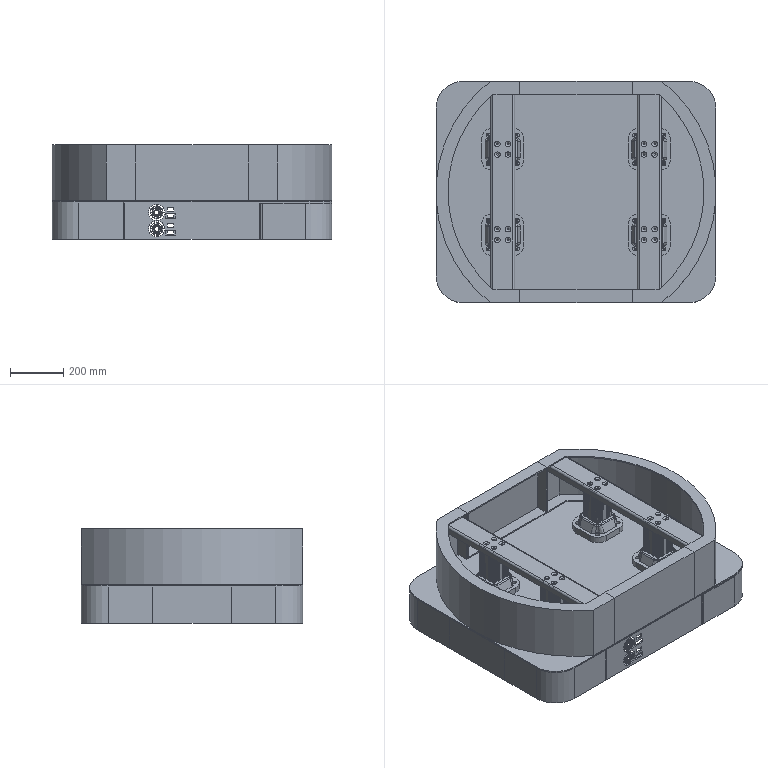Part | NX | features BREP 3 | 32 solids | 3381 faces | volume 24692176 mm3 | plane 2280 | cylinder 943 | spline 64 | torus 48 | cone 32 | sphere 14 | commonest cylinder face diameters 0.6 x128 1 x128 2 x128 6.8 x80 4 x70 10 x38